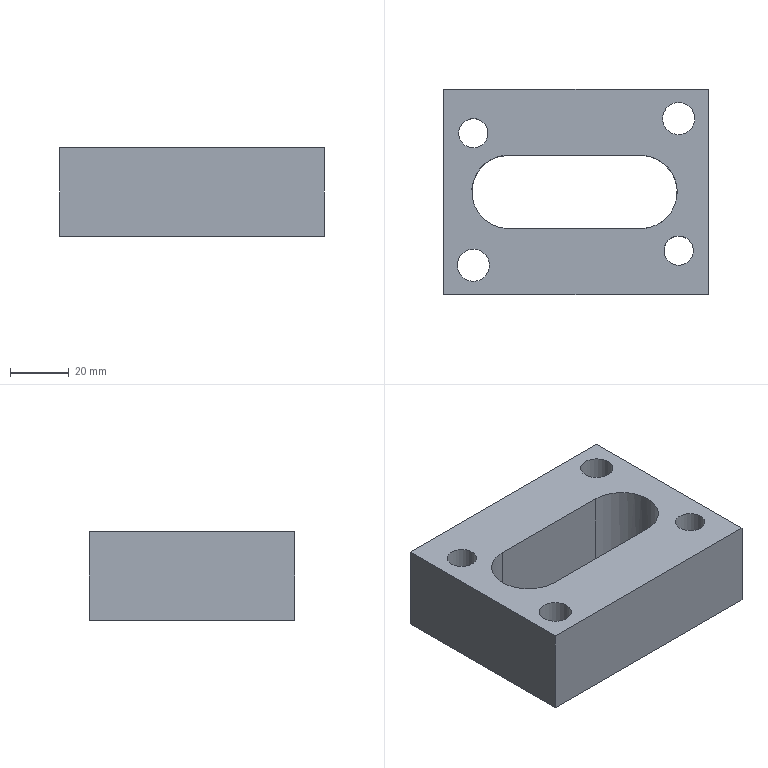Part | NX | features solid 2 | 1 solid | 18 faces | box 90 x 70 x 30 mm | volume 124294 mm3 | plane 10 | cylinder 6 | spline 2 | commonest cylinder face diameters 10 x2 11 x2 17.5 x2
STEP:
#1=CARTESIAN_POINT('',(610.,80.,20.));
#2=VERTEX_POINT('',#1);
#3=CARTESIAN_POINT('',(610.,10.,20.));
#4=VERTEX_POINT('',#3);
#5=CARTESIAN_POINT('',(610.,80.,20.));
#6=DIRECTION('',(0.,-1.,0.));
#7=VECTOR('',#6,1000.);
#8=LINE('',#5,#7);
#9=EDGE_CURVE('',#2,#4,#8,.T.);
#10=ORIENTED_EDGE('',*,*,#9,.F.);
#11=CARTESIAN_POINT('',(610.,80.,50.));
#12=VERTEX_POINT('',#11);
#13=CARTESIAN_POINT('',(610.,80.,50.));
#14=DIRECTION('',(0.,0.,-1.));
#15=VECTOR('',#14,1000.);
#16=LINE('',#13,#15);
#17=EDGE_CURVE('',#12,#2,#16,.T.);
#18=ORIENTED_EDGE('',*,*,#17,.F.);
#19=CARTESIAN_POINT('',(610.,10.,50.));
#20=VERTEX_POINT('',#19);
#21=CARTESIAN_POINT('',(610.,80.,50.));
#22=DIRECTION('',(0.,-1.,0.));
#23=VECTOR('',#22,1000.);
#24=LINE('',#21,#23);
#25=EDGE_CURVE('',#12,#20,#24,.T.);
#26=ORIENTED_EDGE('',*,*,#25,.T.);
#27=CARTESIAN_POINT('',(610.,10.,50.));
#28=DIRECTION('',(0.,0.,-1.));
#29=VECTOR('',#28,1000.);
#30=LINE('',#27,#29);
#31=EDGE_CURVE('',#20,#4,#30,.T.);
#32=ORIENTED_EDGE('',*,*,#31,.T.);
#33=EDGE_LOOP('',(#10,#18,#26,#32));
#34=FACE_BOUND('',#33,.T.);
#35=CARTESIAN_POINT('',(610.,80.,50.));
#36=DIRECTION('',(1.,0.,0.));
#37=DIRECTION('',(0.,0.,-1.));
#38=AXIS2_PLACEMENT_3D('',#35,#36,#37);
#39=PLANE('',#38);
#40=ADVANCED_FACE('',(#34),#39,.T.);
#41=CARTESIAN_POINT('',(520.,10.,20.));
#42=VERTEX_POINT('',#41);
#43=CARTESIAN_POINT('',(610.,10.,20.));
#44=DIRECTION('',(-1.,0.,0.));
#45=VECTOR('',#44,1000.);
#46=LINE('',#43,#45);
#47=EDGE_CURVE('',#4,#42,#46,.T.);
#48=ORIENTED_EDGE('',*,*,#47,.F.);
#49=ORIENTED_EDGE('',*,*,#31,.F.);
#50=CARTESIAN_POINT('',(520.,10.,50.));
#51=VERTEX_POINT('',#50);
#52=CARTESIAN_POINT('',(610.,10.,50.));
#53=DIRECTION('',(-1.,0.,0.));
#54=VECTOR('',#53,1000.);
#55=LINE('',#52,#54);
#56=EDGE_CURVE('',#20,#51,#55,.T.);
#57=ORIENTED_EDGE('',*,*,#56,.T.);
#58=CARTESIAN_POINT('',(520.,10.,50.));
#59=DIRECTION('',(0.,0.,-1.));
#60=VECTOR('',#59,1000.);
#61=LINE('',#58,#60);
#62=EDGE_CURVE('',#51,#42,#61,.T.);
#63=ORIENTED_EDGE('',*,*,#62,.T.);
#64=EDGE_LOOP('',(#48,#49,#57,#63));
#65=FACE_BOUND('',#64,.T.);
#66=CARTESIAN_POINT('',(610.,10.,50.));
#67=DIRECTION('',(0.,-1.,0.));
#68=DIRECTION('',(0.,0.,-1.));
#69=AXIS2_PLACEMENT_3D('',#66,#67,#68);
#70=PLANE('',#69);
#71=ADVANCED_FACE('',(#65),#70,.T.);
#72=CARTESIAN_POINT('',(520.,80.,20.));
#73=VERTEX_POINT('',#72);
#74=CARTESIAN_POINT('',(520.,10.,20.));
#75=DIRECTION('',(0.,1.,0.));
#76=VECTOR('',#75,1000.);
#77=LINE('',#74,#76);
#78=EDGE_CURVE('',#42,#73,#77,.T.);
#79=ORIENTED_EDGE('',*,*,#78,.F.);
#80=ORIENTED_EDGE('',*,*,#62,.F.);
#81=CARTESIAN_POINT('',(520.,80.,50.));
#82=VERTEX_POINT('',#81);
#83=CARTESIAN_POINT('',(520.,10.,50.));
#84=DIRECTION('',(0.,1.,0.));
#85=VECTOR('',#84,1000.);
#86=LINE('',#83,#85);
#87=EDGE_CURVE('',#51,#82,#86,.T.);
#88=ORIENTED_EDGE('',*,*,#87,.T.);
#89=CARTESIAN_POINT('',(520.,80.,50.));
#90=DIRECTION('',(0.,0.,-1.));
#91=VECTOR('',#90,1000.);
#92=LINE('',#89,#91);
#93=EDGE_CURVE('',#82,#73,#92,.T.);
#94=ORIENTED_EDGE('',*,*,#93,.T.);
#95=EDGE_LOOP('',(#79,#80,#88,#94));
#96=FACE_BOUND('',#95,.T.);
#97=CARTESIAN_POINT('',(520.,10.,50.));
#98=DIRECTION('',(-1.,0.,0.));
#99=DIRECTION('',(0.,0.,1.));
#100=AXIS2_PLACEMENT_3D('',#97,#98,#99);
#101=PLANE('',#100);
#102=ADVANCED_FACE('',(#96),#101,.T.);
#103=CARTESIAN_POINT('',(520.,80.,20.));
#104=DIRECTION('',(1.,0.,0.));
#105=VECTOR('',#104,1000.);
#106=LINE('',#103,#105);
#107=EDGE_CURVE('',#73,#2,#106,.T.);
#108=ORIENTED_EDGE('',*,*,#107,.F.);
#109=ORIENTED_EDGE('',*,*,#93,.F.);
#110=CARTESIAN_POINT('',(520.,80.,50.));
#111=DIRECTION('',(1.,0.,0.));
#112=VECTOR('',#111,1000.);
#113=LINE('',#110,#112);
#114=EDGE_CURVE('',#82,#12,#113,.T.);
#115=ORIENTED_EDGE('',*,*,#114,.T.);
#116=ORIENTED_EDGE('',*,*,#17,.T.);
#117=EDGE_LOOP('',(#108,#109,#115,#116));
#118=FACE_BOUND('',#117,.T.);
#119=CARTESIAN_POINT('',(520.,80.,50.));
#120=DIRECTION('',(0.,1.,0.));
#121=DIRECTION('',(0.,0.,1.));
#122=AXIS2_PLACEMENT_3D('',#119,#120,#121);
#123=PLANE('',#122);
#124=ADVANCED_FACE('',(#118),#123,.T.);
#125=CARTESIAN_POINT('',(525.,65.,50.));
#126=VERTEX_POINT('',#125);
#127=CARTESIAN_POINT('',(530.,65.,50.));
#128=DIRECTION('',(0.,0.,-1.));
#129=DIRECTION('',(-1.,0.,0.));
#130=AXIS2_PLACEMENT_3D('',#127,#128,#129);
#131=CIRCLE('',#130,5.);
#132=EDGE_CURVE('',#126,#126,#131,.T.);
#133=ORIENTED_EDGE('',*,*,#132,.T.);
#134=EDGE_LOOP('',(#133));
#135=FACE_BOUND('',#134,.T.);
#136=CARTESIAN_POINT('',(595.,25.,50.));
#137=VERTEX_POINT('',#136);
#138=CARTESIAN_POINT('',(600.,25.,50.));
#139=DIRECTION('',(0.,0.,-1.));
#140=DIRECTION('',(-1.,0.,0.));
#141=AXIS2_PLACEMENT_3D('',#138,#139,#140);
#142=CIRCLE('',#141,5.);
#143=EDGE_CURVE('',#137,#137,#142,.T.);
#144=ORIENTED_EDGE('',*,*,#143,.T.);
#145=EDGE_LOOP('',(#144));
#146=FACE_BOUND('',#145,.T.);
#147=CARTESIAN_POINT('',(594.5,70.,50.));
#148=VERTEX_POINT('',#147);
#149=CARTESIAN_POINT('',(600.,70.,50.));
#150=DIRECTION('',(0.,0.,-1.));
#151=DIRECTION('',(-1.,0.,0.));
#152=AXIS2_PLACEMENT_3D('',#149,#150,#151);
#153=CIRCLE('',#152,5.5);
#154=EDGE_CURVE('',#148,#148,#153,.T.);
#155=ORIENTED_EDGE('',*,*,#154,.T.);
#156=EDGE_LOOP('',(#155));
#157=FACE_BOUND('',#156,.T.);
#158=CARTESIAN_POINT('',(524.5,20.,50.));
#159=VERTEX_POINT('',#158);
#160=CARTESIAN_POINT('',(530.,20.,50.));
#161=DIRECTION('',(0.,0.,-1.));
#162=DIRECTION('',(-1.,0.,0.));
#163=AXIS2_PLACEMENT_3D('',#160,#161,#162);
#164=CIRCLE('',#163,5.5);
#165=EDGE_CURVE('',#159,#159,#164,.T.);
#166=ORIENTED_EDGE('',*,*,#165,.T.);
#167=EDGE_LOOP('',(#166));
#168=FACE_BOUND('',#167,.T.);
#169=CARTESIAN_POINT('',(542.,32.5,50.));
#170=VERTEX_POINT('',#169);
#171=CARTESIAN_POINT('',(542.,57.5,50.));
#172=VERTEX_POINT('',#171);
#173=CARTESIAN_POINT('',(542.,32.5,50.));
#174=CARTESIAN_POINT('',(538.695,32.5,50.));
#175=CARTESIAN_POINT('',(532.208,35.198,50.));
#176=CARTESIAN_POINT('',(528.138,44.985,50.));
#177=CARTESIAN_POINT('',(532.193,54.795,50.));
#178=CARTESIAN_POINT('',(538.696,57.5,50.));
#179=CARTESIAN_POINT('',(542.,57.5,50.));
#180=B_SPLINE_CURVE_WITH_KNOTS('',3,(#173,#174,#175,#176,#177,#178,#179),.UNSPECIFIED.,.F.,.F.,(4,1,1,1,4),(0.,0.009769,0.01954,0.02931,0.03908),.UNSPECIFIED.);
#181=EDGE_CURVE('',#170,#172,#180,.T.);
#182=ORIENTED_EDGE('',*,*,#181,.T.);
#183=CARTESIAN_POINT('',(587.,57.5,50.));
#184=VERTEX_POINT('',#183);
#185=CARTESIAN_POINT('',(542.,57.5,50.));
#186=DIRECTION('',(1.,0.,0.));
#187=VECTOR('',#186,1000.);
#188=LINE('',#185,#187);
#189=EDGE_CURVE('',#172,#184,#188,.T.);
#190=ORIENTED_EDGE('',*,*,#189,.T.);
#191=CARTESIAN_POINT('',(587.,32.5,50.));
#192=VERTEX_POINT('',#191);
#193=CARTESIAN_POINT('',(587.,57.5,50.));
#194=CARTESIAN_POINT('',(590.258,57.5,50.));
#195=CARTESIAN_POINT('',(596.809,54.809,50.));
#196=CARTESIAN_POINT('',(600.858,45.002,50.));
#197=CARTESIAN_POINT('',(596.808,35.18,50.));
#198=CARTESIAN_POINT('',(590.24,32.5,50.));
#199=CARTESIAN_POINT('',(587.,32.5,50.));
#200=B_SPLINE_CURVE_WITH_KNOTS('',3,(#193,#194,#195,#196,#197,#198,#199),.UNSPECIFIED.,.F.,.F.,(4,1,1,1,4),(0.06855,0.07833,0.0881,0.09787,0.1076),.UNSPECIFIED.);
#201=EDGE_CURVE('',#184,#192,#200,.T.);
#202=ORIENTED_EDGE('',*,*,#201,.T.);
#203=CARTESIAN_POINT('',(587.,32.5,50.));
#204=DIRECTION('',(-1.,0.,0.));
#205=VECTOR('',#204,1000.);
#206=LINE('',#203,#205);
#207=EDGE_CURVE('',#192,#170,#206,.T.);
#208=ORIENTED_EDGE('',*,*,#207,.T.);
#209=EDGE_LOOP('',(#182,#190,#202,#208));
#210=FACE_BOUND('',#209,.T.);
#211=ORIENTED_EDGE('',*,*,#25,.F.);
#212=ORIENTED_EDGE('',*,*,#114,.F.);
#213=ORIENTED_EDGE('',*,*,#87,.F.);
#214=ORIENTED_EDGE('',*,*,#56,.F.);
#215=EDGE_LOOP('',(#211,#212,#213,#214));
#216=FACE_BOUND('',#215,.T.);
#217=CARTESIAN_POINT('',(610.,10.,50.));
#218=DIRECTION('',(0.,0.,-1.));
#219=DIRECTION('',(-1.,0.,0.));
#220=AXIS2_PLACEMENT_3D('',#217,#218,#219);
#221=PLANE('',#220);
#222=ADVANCED_FACE('',(#135,#146,#157,#168,#210,#216),#221,.F.);
#223=CARTESIAN_POINT('',(535.,65.,20.));
#224=VERTEX_POINT('',#223);
#225=CARTESIAN_POINT('',(530.,65.,20.));
#226=DIRECTION('',(0.,0.,1.));
#227=DIRECTION('',(1.,0.,0.));
#228=AXIS2_PLACEMENT_3D('',#225,#226,#227);
#229=CIRCLE('',#228,5.);
#230=EDGE_CURVE('',#224,#224,#229,.T.);
#231=ORIENTED_EDGE('',*,*,#230,.T.);
#232=EDGE_LOOP('',(#231));
#233=FACE_BOUND('',#232,.T.);
#234=CARTESIAN_POINT('',(605.,25.,20.));
#235=VERTEX_POINT('',#234);
#236=CARTESIAN_POINT('',(600.,25.,20.));
#237=DIRECTION('',(0.,0.,1.));
#238=DIRECTION('',(1.,0.,0.));
#239=AXIS2_PLACEMENT_3D('',#236,#237,#238);
#240=CIRCLE('',#239,5.);
#241=EDGE_CURVE('',#235,#235,#240,.T.);
#242=ORIENTED_EDGE('',*,*,#241,.T.);
#243=EDGE_LOOP('',(#242));
#244=FACE_BOUND('',#243,.T.);
#245=CARTESIAN_POINT('',(608.75,70.,20.));
#246=VERTEX_POINT('',#245);
#247=CARTESIAN_POINT('',(600.,70.,20.));
#248=DIRECTION('',(0.,0.,1.));
#249=DIRECTION('',(1.,0.,0.));
#250=AXIS2_PLACEMENT_3D('',#247,#248,#249);
#251=CIRCLE('',#250,8.75);
#252=EDGE_CURVE('',#246,#246,#251,.T.);
#253=ORIENTED_EDGE('',*,*,#252,.T.);
#254=EDGE_LOOP('',(#253));
#255=FACE_BOUND('',#254,.T.);
#256=CARTESIAN_POINT('',(538.75,20.,20.));
#257=VERTEX_POINT('',#256);
#258=CARTESIAN_POINT('',(530.,20.,20.));
#259=DIRECTION('',(0.,0.,1.));
#260=DIRECTION('',(1.,0.,0.));
#261=AXIS2_PLACEMENT_3D('',#258,#259,#260);
#262=CIRCLE('',#261,8.75);
#263=EDGE_CURVE('',#257,#257,#262,.T.);
#264=ORIENTED_EDGE('',*,*,#263,.T.);
#265=EDGE_LOOP('',(#264));
#266=FACE_BOUND('',#265,.T.);
#267=CARTESIAN_POINT('',(542.,57.5,20.));
#268=VERTEX_POINT('',#267);
#269=CARTESIAN_POINT('',(587.,57.5,20.));
#270=VERTEX_POINT('',#269);
#271=CARTESIAN_POINT('',(610.,57.5,20.));
#272=DIRECTION('',(1.,0.,0.));
#273=VECTOR('',#272,1000.);
#274=LINE('',#271,#273);
#275=EDGE_CURVE('',#268,#270,#274,.T.);
#276=ORIENTED_EDGE('',*,*,#275,.F.);
#277=CARTESIAN_POINT('',(542.,32.5,20.));
#278=VERTEX_POINT('',#277);
#279=CARTESIAN_POINT('',(542.,32.5,20.));
#280=CARTESIAN_POINT('',(540.362,32.5,20.));
#281=CARTESIAN_POINT('',(537.095,33.167,20.));
#282=CARTESIAN_POINT('',(532.914,35.916,20.));
#283=CARTESIAN_POINT('',(530.163,40.093,20.));
#284=CARTESIAN_POINT('',(529.157,45.,20.));
#285=CARTESIAN_POINT('',(530.163,49.907,20.));
#286=CARTESIAN_POINT('',(532.914,54.084,20.));
#287=CARTESIAN_POINT('',(537.095,56.833,20.));
#288=CARTESIAN_POINT('',(540.362,57.5,20.));
#289=CARTESIAN_POINT('',(542.,57.5,20.));
#290=B_SPLINE_CURVE_WITH_KNOTS('',3,(#279,#280,#281,#282,#283,#284,#285,#286,#287,#288,#289),.UNSPECIFIED.,.F.,.F.,(4,1,1,1,1,1,1,1,4),(0.,0.125,0.25,0.375,0.5,0.625,0.75,0.875,1.),.QUASI_UNIFORM_KNOTS.);
#291=EDGE_CURVE('',#278,#268,#290,.T.);
#292=ORIENTED_EDGE('',*,*,#291,.F.);
#293=CARTESIAN_POINT('',(587.,32.5,20.));
#294=VERTEX_POINT('',#293);
#295=CARTESIAN_POINT('',(610.,32.5,20.));
#296=DIRECTION('',(-1.,0.,0.));
#297=VECTOR('',#296,1000.);
#298=LINE('',#295,#297);
#299=EDGE_CURVE('',#294,#278,#298,.T.);
#300=ORIENTED_EDGE('',*,*,#299,.F.);
#301=CARTESIAN_POINT('',(587.,57.5,20.));
#302=CARTESIAN_POINT('',(588.638,57.5,20.));
#303=CARTESIAN_POINT('',(591.905,56.833,20.));
#304=CARTESIAN_POINT('',(596.086,54.084,20.));
#305=CARTESIAN_POINT('',(598.837,49.907,20.));
#306=CARTESIAN_POINT('',(599.843,45.,20.));
#307=CARTESIAN_POINT('',(598.837,40.093,20.));
#308=CARTESIAN_POINT('',(596.086,35.916,20.));
#309=CARTESIAN_POINT('',(591.905,33.167,20.));
#310=CARTESIAN_POINT('',(588.638,32.5,20.));
#311=CARTESIAN_POINT('',(587.,32.5,20.));
#312=B_SPLINE_CURVE_WITH_KNOTS('',3,(#301,#302,#303,#304,#305,#306,#307,#308,#309,#310,#311),.UNSPECIFIED.,.F.,.F.,(4,1,1,1,1,1,1,1,4),(0.,0.125,0.25,0.375,0.5,0.625,0.75,0.875,1.),.QUASI_UNIFORM_KNOTS.);
#313=EDGE_CURVE('',#270,#294,#312,.T.);
#314=ORIENTED_EDGE('',*,*,#313,.F.);
#315=EDGE_LOOP('',(#276,#292,#300,#314));
#316=FACE_BOUND('',#315,.T.);
#317=ORIENTED_EDGE('',*,*,#9,.T.);
#318=ORIENTED_EDGE('',*,*,#47,.T.);
#319=ORIENTED_EDGE('',*,*,#78,.T.);
#320=ORIENTED_EDGE('',*,*,#107,.T.);
#321=EDGE_LOOP('',(#317,#318,#319,#320));
#322=FACE_BOUND('',#321,.T.);
#323=CARTESIAN_POINT('',(610.,10.,20.));
#324=DIRECTION('',(0.,0.,-1.));
#325=DIRECTION('',(-1.,0.,0.));
#326=AXIS2_PLACEMENT_3D('',#323,#324,#325);
#327=PLANE('',#326);
#328=ADVANCED_FACE('',(#233,#244,#255,#266,#316,#322),#327,.T.);
#329=ORIENTED_EDGE('',*,*,#275,.T.);
#330=CARTESIAN_POINT('',(587.,57.5,20.));
#331=DIRECTION('',(0.,0.,-1.));
#332=VECTOR('',#331,1000.);
#333=LINE('',#330,#332);
#334=EDGE_CURVE('',#184,#270,#333,.T.);
#335=ORIENTED_EDGE('',*,*,#334,.F.);
#336=ORIENTED_EDGE('',*,*,#189,.F.);
#337=CARTESIAN_POINT('',(542.,57.5,20.));
#338=DIRECTION('',(0.,0.,-1.));
#339=VECTOR('',#338,1000.);
#340=LINE('',#337,#339);
#341=EDGE_CURVE('',#172,#268,#340,.T.);
#342=ORIENTED_EDGE('',*,*,#341,.T.);
#343=EDGE_LOOP('',(#329,#335,#336,#342));
#344=FACE_BOUND('',#343,.T.);
#345=CARTESIAN_POINT('',(542.,57.5,20.));
#346=DIRECTION('',(0.,1.,0.));
#347=DIRECTION('',(0.,0.,1.));
#348=AXIS2_PLACEMENT_3D('',#345,#346,#347);
#349=PLANE('',#348);
#350=ADVANCED_FACE('',(#344),#349,.F.);
#351=ORIENTED_EDGE('',*,*,#313,.T.);
#352=CARTESIAN_POINT('',(587.,32.5,20.));
#353=DIRECTION('',(0.,0.,-1.));
#354=VECTOR('',#353,1000.);
#355=LINE('',#352,#354);
#356=EDGE_CURVE('',#192,#294,#355,.T.);
#357=ORIENTED_EDGE('',*,*,#356,.F.);
#358=ORIENTED_EDGE('',*,*,#201,.F.);
#359=ORIENTED_EDGE('',*,*,#334,.T.);
#360=EDGE_LOOP('',(#351,#357,#358,#359));
#361=FACE_BOUND('',#360,.T.);
#362=CARTESIAN_POINT('',(587.,57.5,50.));
#363=CARTESIAN_POINT('',(587.,57.5,20.));
#364=CARTESIAN_POINT('',(590.276,57.5,50.));
#365=CARTESIAN_POINT('',(590.276,57.5,20.));
#366=CARTESIAN_POINT('',(596.803,54.807,50.));
#367=CARTESIAN_POINT('',(596.803,54.807,20.));
#368=CARTESIAN_POINT('',(600.86,45.,50.));
#369=CARTESIAN_POINT('',(600.86,45.,20.));
#370=CARTESIAN_POINT('',(596.803,35.193,50.));
#371=CARTESIAN_POINT('',(596.803,35.193,20.));
#372=CARTESIAN_POINT('',(590.276,32.5,50.));
#373=CARTESIAN_POINT('',(590.276,32.5,20.));
#374=CARTESIAN_POINT('',(587.,32.5,50.));
#375=CARTESIAN_POINT('',(587.,32.5,20.));
#376=B_SPLINE_SURFACE_WITH_KNOTS('',3,1,((#362,#363),(#364,#365),(#366,#367),(#368,#369),(#370,#371),(#372,#373),(#374,#375)),.SURF_OF_LINEAR_EXTRUSION.,.F.,.F.,.F.,(4,1,1,1,4),(2,2),(0.,0.25,0.5,0.75,1.),(0.,1.),.UNSPECIFIED.);
#377=ADVANCED_FACE('',(#361),#376,.F.);
#378=ORIENTED_EDGE('',*,*,#299,.T.);
#379=CARTESIAN_POINT('',(542.,32.5,20.));
#380=DIRECTION('',(0.,0.,-1.));
#381=VECTOR('',#380,1000.);
#382=LINE('',#379,#381);
#383=EDGE_CURVE('',#170,#278,#382,.T.);
#384=ORIENTED_EDGE('',*,*,#383,.F.);
#385=ORIENTED_EDGE('',*,*,#207,.F.);
#386=ORIENTED_EDGE('',*,*,#356,.T.);
#387=EDGE_LOOP('',(#378,#384,#385,#386));
#388=FACE_BOUND('',#387,.T.);
#389=CARTESIAN_POINT('',(587.,32.5,20.));
#390=DIRECTION('',(0.,-1.,0.));
#391=DIRECTION('',(0.,0.,-1.));
#392=AXIS2_PLACEMENT_3D('',#389,#390,#391);
#393=PLANE('',#392);
#394=ADVANCED_FACE('',(#388),#393,.F.);
#395=ORIENTED_EDGE('',*,*,#291,.T.);
#396=ORIENTED_EDGE('',*,*,#341,.F.);
#397=ORIENTED_EDGE('',*,*,#181,.F.);
#398=ORIENTED_EDGE('',*,*,#383,.T.);
#399=EDGE_LOOP('',(#395,#396,#397,#398));
#400=FACE_BOUND('',#399,.T.);
#401=CARTESIAN_POINT('',(542.,32.5,50.));
#402=CARTESIAN_POINT('',(542.,32.5,20.));
#403=CARTESIAN_POINT('',(538.724,32.5,50.));
#404=CARTESIAN_POINT('',(538.724,32.5,20.));
#405=CARTESIAN_POINT('',(532.197,35.193,50.));
#406=CARTESIAN_POINT('',(532.197,35.193,20.));
#407=CARTESIAN_POINT('',(528.14,45.,50.));
#408=CARTESIAN_POINT('',(528.14,45.,20.));
#409=CARTESIAN_POINT('',(532.197,54.807,50.));
#410=CARTESIAN_POINT('',(532.197,54.807,20.));
#411=CARTESIAN_POINT('',(538.724,57.5,50.));
#412=CARTESIAN_POINT('',(538.724,57.5,20.));
#413=CARTESIAN_POINT('',(542.,57.5,50.));
#414=CARTESIAN_POINT('',(542.,57.5,20.));
#415=B_SPLINE_SURFACE_WITH_KNOTS('',3,1,((#401,#402),(#403,#404),(#405,#406),(#407,#408),(#409,#410),(#411,#412),(#413,#414)),.SURF_OF_LINEAR_EXTRUSION.,.F.,.F.,.F.,(4,1,1,1,4),(2,2),(0.,0.25,0.5,0.75,1.),(0.,1.),.UNSPECIFIED.);
#416=ADVANCED_FACE('',(#400),#415,.F.);
#417=CARTESIAN_POINT('',(535.5,20.,40.));
#418=VERTEX_POINT('',#417);
#419=CARTESIAN_POINT('',(530.,20.,40.));
#420=DIRECTION('',(0.,0.,1.));
#421=DIRECTION('',(1.,0.,0.));
#422=AXIS2_PLACEMENT_3D('',#419,#420,#421);
#423=CIRCLE('',#422,5.5);
#424=EDGE_CURVE('',#418,#418,#423,.T.);
#425=ORIENTED_EDGE('',*,*,#424,.F.);
#426=EDGE_LOOP('',(#425));
#427=FACE_BOUND('',#426,.T.);
#428=ORIENTED_EDGE('',*,*,#165,.F.);
#429=EDGE_LOOP('',(#428));
#430=FACE_BOUND('',#429,.T.);
#431=CARTESIAN_POINT('',(530.,20.,70.));
#432=DIRECTION('',(0.,0.,1.));
#433=DIRECTION('',(1.,0.,0.));
#434=AXIS2_PLACEMENT_3D('',#431,#432,#433);
#435=CYLINDRICAL_SURFACE('',#434,5.5);
#436=ADVANCED_FACE('',(#427,#430),#435,.F.);
#437=ORIENTED_EDGE('',*,*,#424,.T.);
#438=EDGE_LOOP('',(#437));
#439=FACE_BOUND('',#438,.T.);
#440=CARTESIAN_POINT('',(538.75,20.,40.));
#441=VERTEX_POINT('',#440);
#442=CARTESIAN_POINT('',(530.,20.,40.));
#443=DIRECTION('',(0.,0.,1.));
#444=DIRECTION('',(1.,0.,0.));
#445=AXIS2_PLACEMENT_3D('',#442,#443,#444);
#446=CIRCLE('',#445,8.75);
#447=EDGE_CURVE('',#441,#441,#446,.T.);
#448=ORIENTED_EDGE('',*,*,#447,.F.);
#449=EDGE_LOOP('',(#448));
#450=FACE_BOUND('',#449,.T.);
#451=CARTESIAN_POINT('',(530.,20.,40.));
#452=DIRECTION('',(0.,0.,1.));
#453=DIRECTION('',(1.,0.,0.));
#454=AXIS2_PLACEMENT_3D('',#451,#452,#453);
#455=PLANE('',#454);
#456=ADVANCED_FACE('',(#439,#450),#455,.F.);
#457=ORIENTED_EDGE('',*,*,#447,.T.);
#458=EDGE_LOOP('',(#457));
#459=FACE_BOUND('',#458,.T.);
#460=ORIENTED_EDGE('',*,*,#263,.F.);
#461=EDGE_LOOP('',(#460));
#462=FACE_BOUND('',#461,.T.);
#463=CARTESIAN_POINT('',(530.,20.,20.));
#464=DIRECTION('',(0.,0.,1.));
#465=DIRECTION('',(1.,0.,0.));
#466=AXIS2_PLACEMENT_3D('',#463,#464,#465);
#467=CYLINDRICAL_SURFACE('',#466,8.75);
#468=ADVANCED_FACE('',(#459,#462),#467,.F.);
#469=CARTESIAN_POINT('',(605.5,70.,40.));
#470=VERTEX_POINT('',#469);
#471=CARTESIAN_POINT('',(600.,70.,40.));
#472=DIRECTION('',(0.,0.,1.));
#473=DIRECTION('',(1.,0.,0.));
#474=AXIS2_PLACEMENT_3D('',#471,#472,#473);
#475=CIRCLE('',#474,5.5);
#476=EDGE_CURVE('',#470,#470,#475,.T.);
#477=ORIENTED_EDGE('',*,*,#476,.F.);
#478=EDGE_LOOP('',(#477));
#479=FACE_BOUND('',#478,.T.);
#480=ORIENTED_EDGE('',*,*,#154,.F.);
#481=EDGE_LOOP('',(#480));
#482=FACE_BOUND('',#481,.T.);
#483=CARTESIAN_POINT('',(600.,70.,70.));
#484=DIRECTION('',(0.,0.,1.));
#485=DIRECTION('',(1.,0.,0.));
#486=AXIS2_PLACEMENT_3D('',#483,#484,#485);
#487=CYLINDRICAL_SURFACE('',#486,5.5);
#488=ADVANCED_FACE('',(#479,#482),#487,.F.);
#489=ORIENTED_EDGE('',*,*,#476,.T.);
#490=EDGE_LOOP('',(#489));
#491=FACE_BOUND('',#490,.T.);
#492=CARTESIAN_POINT('',(608.75,70.,40.));
#493=VERTEX_POINT('',#492);
#494=CARTESIAN_POINT('',(600.,70.,40.));
#495=DIRECTION('',(0.,0.,1.));
#496=DIRECTION('',(1.,0.,0.));
#497=AXIS2_PLACEMENT_3D('',#494,#495,#496);
#498=CIRCLE('',#497,8.75);
#499=EDGE_CURVE('',#493,#493,#498,.T.);
#500=ORIENTED_EDGE('',*,*,#499,.F.);
#501=EDGE_LOOP('',(#500));
#502=FACE_BOUND('',#501,.T.);
#503=CARTESIAN_POINT('',(600.,70.,40.));
#504=DIRECTION('',(0.,0.,1.));
#505=DIRECTION('',(1.,0.,0.));
#506=AXIS2_PLACEMENT_3D('',#503,#504,#505);
#507=PLANE('',#506);
#508=ADVANCED_FACE('',(#491,#502),#507,.F.);
#509=ORIENTED_EDGE('',*,*,#499,.T.);
#510=EDGE_LOOP('',(#509));
#511=FACE_BOUND('',#510,.T.);
#512=ORIENTED_EDGE('',*,*,#252,.F.);
#513=EDGE_LOOP('',(#512));
#514=FACE_BOUND('',#513,.T.);
#515=CARTESIAN_POINT('',(600.,70.,20.));
#516=DIRECTION('',(0.,0.,1.));
#517=DIRECTION('',(1.,0.,0.));
#518=AXIS2_PLACEMENT_3D('',#515,#516,#517);
#519=CYLINDRICAL_SURFACE('',#518,8.75);
#520=ADVANCED_FACE('',(#511,#514),#519,.F.);
#521=ORIENTED_EDGE('',*,*,#241,.F.);
#522=EDGE_LOOP('',(#521));
#523=FACE_BOUND('',#522,.T.);
#524=ORIENTED_EDGE('',*,*,#143,.F.);
#525=EDGE_LOOP('',(#524));
#526=FACE_BOUND('',#525,.T.);
#527=CARTESIAN_POINT('',(600.,25.,20.));
#528=DIRECTION('',(0.,0.,1.));
#529=DIRECTION('',(1.,0.,0.));
#530=AXIS2_PLACEMENT_3D('',#527,#528,#529);
#531=CYLINDRICAL_SURFACE('',#530,5.);
#532=ADVANCED_FACE('',(#523,#526),#531,.F.);
#533=ORIENTED_EDGE('',*,*,#230,.F.);
#534=EDGE_LOOP('',(#533));
#535=FACE_BOUND('',#534,.T.);
#536=ORIENTED_EDGE('',*,*,#132,.F.);
#537=EDGE_LOOP('',(#536));
#538=FACE_BOUND('',#537,.T.);
#539=CARTESIAN_POINT('',(530.,65.,20.));
#540=DIRECTION('',(0.,0.,1.));
#541=DIRECTION('',(1.,0.,0.));
#542=AXIS2_PLACEMENT_3D('',#539,#540,#541);
#543=CYLINDRICAL_SURFACE('',#542,5.);
#544=ADVANCED_FACE('',(#535,#538),#543,.F.);
#545=CLOSED_SHELL('',(#40,#71,#102,#124,#222,#328,#350,#377,#394,#416,#436,#456,#468,#488,#508,#520,#532,#544));
#546=MANIFOLD_SOLID_BREP('',#545);
#547=(LENGTH_UNIT()NAMED_UNIT(*)SI_UNIT(.MILLI.,.METRE.));
#548=UNCERTAINTY_MEASURE_WITH_UNIT(LENGTH_MEASURE(0.0508),#547,'','');
#549=(NAMED_UNIT(*)PLANE_ANGLE_UNIT()SI_UNIT($,.RADIAN.));
#550=(NAMED_UNIT(*)SI_UNIT($,.STERADIAN.)SOLID_ANGLE_UNIT());
#551=(GEOMETRIC_REPRESENTATION_CONTEXT(3)GLOBAL_UNCERTAINTY_ASSIGNED_CONTEXT((#548))GLOBAL_UNIT_ASSIGNED_CONTEXT((#547,#549,#550))REPRESENTATION_CONTEXT('',''));
#552=ADVANCED_BREP_SHAPE_REPRESENTATION('',(#546),#551);